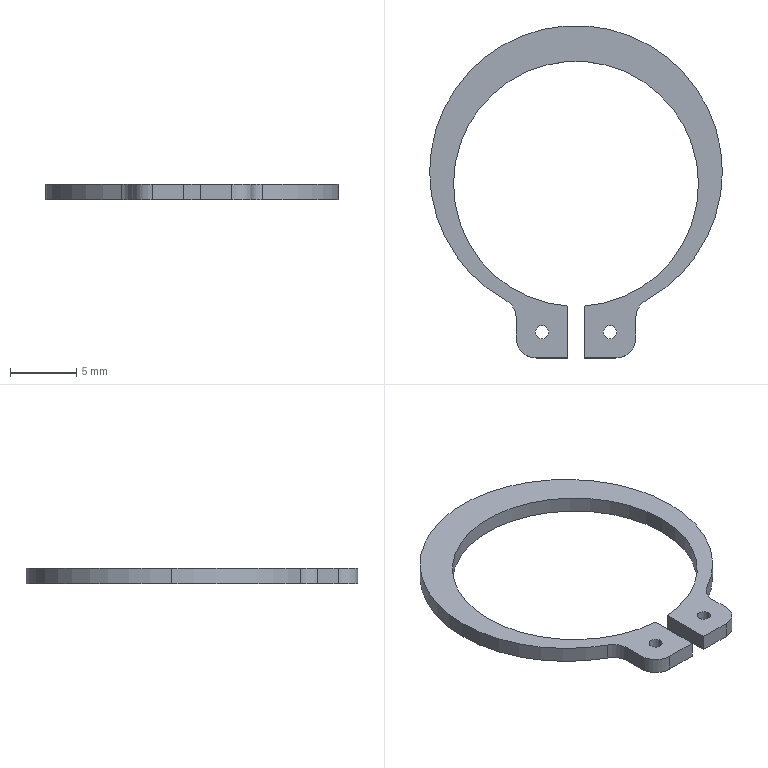Part | NX | features BREP 1 | 1 solid | 22 faces | box 22.1 x 25.1 x 1.2 mm | volume 165.202 mm3 | cylinder 14 | plane 8 | commonest cylinder face diameters 1 x4 3.011 x4 18.5 x3 22.1 x3
STEP:
#1=CARTESIAN_POINT('',(-3.067,-11.2,0.6));
#2=VERTEX_POINT('',#1);
#3=CARTESIAN_POINT('',(-2.067,-11.2,0.6));
#4=VERTEX_POINT('',#3);
#5=CARTESIAN_POINT('',(-2.567,-11.2,0.6));
#6=DIRECTION('',(0.,0.,1.));
#7=DIRECTION('',(1.,0.,0.));
#8=AXIS2_PLACEMENT_3D('',#5,#6,#7);
#9=CIRCLE('',#8,0.5);
#10=EDGE_CURVE('',#2,#4,#9,.T.);
#11=ORIENTED_EDGE('',*,*,#10,.T.);
#12=CARTESIAN_POINT('',(-2.067,-11.2,-0.6));
#13=VERTEX_POINT('',#12);
#14=CARTESIAN_POINT('',(-2.067,-11.2,0.6));
#15=DIRECTION('',(0.,0.,-1.));
#16=VECTOR('',#15,1000.);
#17=LINE('',#14,#16);
#18=EDGE_CURVE('',#13,#4,#17,.F.);
#19=ORIENTED_EDGE('',*,*,#18,.F.);
#20=CARTESIAN_POINT('',(-3.067,-11.2,-0.6));
#21=VERTEX_POINT('',#20);
#22=CARTESIAN_POINT('',(-2.567,-11.2,-0.6));
#23=DIRECTION('',(0.,0.,1.));
#24=DIRECTION('',(1.,0.,0.));
#25=AXIS2_PLACEMENT_3D('',#22,#23,#24);
#26=CIRCLE('',#25,0.5);
#27=EDGE_CURVE('',#21,#13,#26,.T.);
#28=ORIENTED_EDGE('',*,*,#27,.F.);
#29=CARTESIAN_POINT('',(-3.067,-11.2,0.6));
#30=DIRECTION('',(0.,0.,-1.));
#31=VECTOR('',#30,1000.);
#32=LINE('',#29,#31);
#33=EDGE_CURVE('',#21,#2,#32,.F.);
#34=ORIENTED_EDGE('',*,*,#33,.T.);
#35=EDGE_LOOP('',(#11,#19,#28,#34));
#36=FACE_BOUND('',#35,.T.);
#37=CARTESIAN_POINT('',(-2.567,-11.2,0.6));
#38=DIRECTION('',(0.,0.,-1.));
#39=DIRECTION('',(1.,0.,0.));
#40=AXIS2_PLACEMENT_3D('',#37,#38,#39);
#41=CYLINDRICAL_SURFACE('',#40,0.5);
#42=ADVANCED_FACE('',(#36),#41,.F.);
#43=CARTESIAN_POINT('',(2.067,-11.2,0.6));
#44=VERTEX_POINT('',#43);
#45=CARTESIAN_POINT('',(3.067,-11.2,0.6));
#46=VERTEX_POINT('',#45);
#47=CARTESIAN_POINT('',(2.567,-11.2,0.6));
#48=DIRECTION('',(0.,0.,1.));
#49=DIRECTION('',(1.,0.,0.));
#50=AXIS2_PLACEMENT_3D('',#47,#48,#49);
#51=CIRCLE('',#50,0.5);
#52=EDGE_CURVE('',#44,#46,#51,.T.);
#53=ORIENTED_EDGE('',*,*,#52,.T.);
#54=CARTESIAN_POINT('',(3.067,-11.2,-0.6));
#55=VERTEX_POINT('',#54);
#56=CARTESIAN_POINT('',(3.067,-11.2,0.6));
#57=DIRECTION('',(0.,0.,-1.));
#58=VECTOR('',#57,1000.);
#59=LINE('',#56,#58);
#60=EDGE_CURVE('',#55,#46,#59,.F.);
#61=ORIENTED_EDGE('',*,*,#60,.F.);
#62=CARTESIAN_POINT('',(2.067,-11.2,-0.6));
#63=VERTEX_POINT('',#62);
#64=CARTESIAN_POINT('',(2.567,-11.2,-0.6));
#65=DIRECTION('',(0.,0.,1.));
#66=DIRECTION('',(1.,0.,0.));
#67=AXIS2_PLACEMENT_3D('',#64,#65,#66);
#68=CIRCLE('',#67,0.5);
#69=EDGE_CURVE('',#63,#55,#68,.T.);
#70=ORIENTED_EDGE('',*,*,#69,.F.);
#71=CARTESIAN_POINT('',(2.067,-11.2,0.6));
#72=DIRECTION('',(0.,0.,-1.));
#73=VECTOR('',#72,1000.);
#74=LINE('',#71,#73);
#75=EDGE_CURVE('',#63,#44,#74,.F.);
#76=ORIENTED_EDGE('',*,*,#75,.T.);
#77=EDGE_LOOP('',(#53,#61,#70,#76));
#78=FACE_BOUND('',#77,.T.);
#79=CARTESIAN_POINT('',(2.567,-11.2,0.6));
#80=DIRECTION('',(0.,0.,-1.));
#81=DIRECTION('',(1.,0.,0.));
#82=AXIS2_PLACEMENT_3D('',#79,#80,#81);
#83=CYLINDRICAL_SURFACE('',#82,0.5);
#84=ADVANCED_FACE('',(#78),#83,.F.);
#85=CARTESIAN_POINT('',(9.25,0.,0.6));
#86=VERTEX_POINT('',#85);
#87=CARTESIAN_POINT('',(0.6167,-9.229,0.6));
#88=VERTEX_POINT('',#87);
#89=CARTESIAN_POINT('',(0.,0.,0.6));
#90=DIRECTION('',(0.,0.,-1.));
#91=DIRECTION('',(-1.,0.,0.));
#92=AXIS2_PLACEMENT_3D('',#89,#90,#91);
#93=CIRCLE('',#92,9.25);
#94=EDGE_CURVE('',#86,#88,#93,.T.);
#95=ORIENTED_EDGE('',*,*,#94,.F.);
#96=CARTESIAN_POINT('',(9.25,0.,-0.6));
#97=VERTEX_POINT('',#96);
#98=CARTESIAN_POINT('',(9.25,0.,0.6));
#99=DIRECTION('',(0.,0.,-1.));
#100=VECTOR('',#99,1000.);
#101=LINE('',#98,#100);
#102=EDGE_CURVE('',#86,#97,#101,.T.);
#103=ORIENTED_EDGE('',*,*,#102,.T.);
#104=CARTESIAN_POINT('',(0.6167,-9.229,-0.6));
#105=VERTEX_POINT('',#104);
#106=CARTESIAN_POINT('',(0.,0.,-0.6));
#107=DIRECTION('',(0.,0.,-1.));
#108=DIRECTION('',(-1.,0.,0.));
#109=AXIS2_PLACEMENT_3D('',#106,#107,#108);
#110=CIRCLE('',#109,9.25);
#111=EDGE_CURVE('',#97,#105,#110,.T.);
#112=ORIENTED_EDGE('',*,*,#111,.T.);
#113=CARTESIAN_POINT('',(0.6167,-9.229,0.6));
#114=DIRECTION('',(0.,0.,-1.));
#115=VECTOR('',#114,1000.);
#116=LINE('',#113,#115);
#117=EDGE_CURVE('',#88,#105,#116,.T.);
#118=ORIENTED_EDGE('',*,*,#117,.F.);
#119=EDGE_LOOP('',(#95,#103,#112,#118));
#120=FACE_BOUND('',#119,.T.);
#121=CARTESIAN_POINT('',(0.,0.,0.6));
#122=DIRECTION('',(0.,0.,-1.));
#123=DIRECTION('',(1.,0.,0.));
#124=AXIS2_PLACEMENT_3D('',#121,#122,#123);
#125=CYLINDRICAL_SURFACE('',#124,9.25);
#126=ADVANCED_FACE('',(#120),#125,.F.);
#127=ORIENTED_EDGE('',*,*,#102,.F.);
#128=CARTESIAN_POINT('',(-9.25,0.,0.6));
#129=VERTEX_POINT('',#128);
#130=CARTESIAN_POINT('',(0.,0.,0.6));
#131=DIRECTION('',(0.,0.,-1.));
#132=DIRECTION('',(-1.,0.,0.));
#133=AXIS2_PLACEMENT_3D('',#130,#131,#132);
#134=CIRCLE('',#133,9.25);
#135=EDGE_CURVE('',#129,#86,#134,.T.);
#136=ORIENTED_EDGE('',*,*,#135,.F.);
#137=CARTESIAN_POINT('',(-9.25,0.,-0.6));
#138=VERTEX_POINT('',#137);
#139=CARTESIAN_POINT('',(-9.25,0.,0.6));
#140=DIRECTION('',(0.,0.,-1.));
#141=VECTOR('',#140,1000.);
#142=LINE('',#139,#141);
#143=EDGE_CURVE('',#129,#138,#142,.T.);
#144=ORIENTED_EDGE('',*,*,#143,.T.);
#145=CARTESIAN_POINT('',(0.,0.,-0.6));
#146=DIRECTION('',(0.,0.,-1.));
#147=DIRECTION('',(-1.,0.,0.));
#148=AXIS2_PLACEMENT_3D('',#145,#146,#147);
#149=CIRCLE('',#148,9.25);
#150=EDGE_CURVE('',#138,#97,#149,.T.);
#151=ORIENTED_EDGE('',*,*,#150,.T.);
#152=EDGE_LOOP('',(#127,#136,#144,#151));
#153=FACE_BOUND('',#152,.T.);
#154=CARTESIAN_POINT('',(0.,0.,0.6));
#155=DIRECTION('',(0.,0.,-1.));
#156=DIRECTION('',(1.,0.,0.));
#157=AXIS2_PLACEMENT_3D('',#154,#155,#156);
#158=CYLINDRICAL_SURFACE('',#157,9.25);
#159=ADVANCED_FACE('',(#153),#158,.F.);
#160=CARTESIAN_POINT('',(11.05,0.9,0.6));
#161=VERTEX_POINT('',#160);
#162=CARTESIAN_POINT('',(-11.05,0.9,0.6));
#163=VERTEX_POINT('',#162);
#164=CARTESIAN_POINT('',(0.,0.9,0.6));
#165=DIRECTION('',(0.,0.,1.));
#166=DIRECTION('',(1.,0.,0.));
#167=AXIS2_PLACEMENT_3D('',#164,#165,#166);
#168=CIRCLE('',#167,11.05);
#169=EDGE_CURVE('',#161,#163,#168,.T.);
#170=ORIENTED_EDGE('',*,*,#169,.F.);
#171=CARTESIAN_POINT('',(11.05,0.9,-0.6));
#172=VERTEX_POINT('',#171);
#173=CARTESIAN_POINT('',(11.05,0.9,0.6));
#174=DIRECTION('',(0.,0.,-1.));
#175=VECTOR('',#174,1000.);
#176=LINE('',#173,#175);
#177=EDGE_CURVE('',#161,#172,#176,.T.);
#178=ORIENTED_EDGE('',*,*,#177,.T.);
#179=CARTESIAN_POINT('',(-11.05,0.9,-0.6));
#180=VERTEX_POINT('',#179);
#181=CARTESIAN_POINT('',(0.,0.9,-0.6));
#182=DIRECTION('',(0.,0.,1.));
#183=DIRECTION('',(1.,0.,0.));
#184=AXIS2_PLACEMENT_3D('',#181,#182,#183);
#185=CIRCLE('',#184,11.05);
#186=EDGE_CURVE('',#172,#180,#185,.T.);
#187=ORIENTED_EDGE('',*,*,#186,.T.);
#188=CARTESIAN_POINT('',(-11.05,0.9,0.6));
#189=DIRECTION('',(0.,0.,-1.));
#190=VECTOR('',#189,1000.);
#191=LINE('',#188,#190);
#192=EDGE_CURVE('',#163,#180,#191,.T.);
#193=ORIENTED_EDGE('',*,*,#192,.F.);
#194=EDGE_LOOP('',(#170,#178,#187,#193));
#195=FACE_BOUND('',#194,.T.);
#196=CARTESIAN_POINT('',(0.,0.9,0.6));
#197=DIRECTION('',(0.,0.,-1.));
#198=DIRECTION('',(1.,0.,0.));
#199=AXIS2_PLACEMENT_3D('',#196,#197,#198);
#200=CYLINDRICAL_SURFACE('',#199,11.05);
#201=ADVANCED_FACE('',(#195),#200,.T.);
#202=CARTESIAN_POINT('',(-5.3,-8.796,0.6));
#203=VERTEX_POINT('',#202);
#204=CARTESIAN_POINT('',(0.,0.9,0.6));
#205=DIRECTION('',(0.,0.,1.));
#206=DIRECTION('',(1.,0.,0.));
#207=AXIS2_PLACEMENT_3D('',#204,#205,#206);
#208=CIRCLE('',#207,11.05);
#209=EDGE_CURVE('',#163,#203,#208,.T.);
#210=ORIENTED_EDGE('',*,*,#209,.F.);
#211=ORIENTED_EDGE('',*,*,#192,.T.);
#212=CARTESIAN_POINT('',(-5.3,-8.796,-0.6));
#213=VERTEX_POINT('',#212);
#214=CARTESIAN_POINT('',(0.,0.9,-0.6));
#215=DIRECTION('',(0.,0.,1.));
#216=DIRECTION('',(1.,0.,0.));
#217=AXIS2_PLACEMENT_3D('',#214,#215,#216);
#218=CIRCLE('',#217,11.05);
#219=EDGE_CURVE('',#180,#213,#218,.T.);
#220=ORIENTED_EDGE('',*,*,#219,.T.);
#221=CARTESIAN_POINT('',(-5.3,-8.796,0.6));
#222=DIRECTION('',(0.,0.,-1.));
#223=VECTOR('',#222,1000.);
#224=LINE('',#221,#223);
#225=EDGE_CURVE('',#203,#213,#224,.T.);
#226=ORIENTED_EDGE('',*,*,#225,.F.);
#227=EDGE_LOOP('',(#210,#211,#220,#226));
#228=FACE_BOUND('',#227,.T.);
#229=CARTESIAN_POINT('',(0.,0.9,0.6));
#230=DIRECTION('',(0.,0.,-1.));
#231=DIRECTION('',(1.,0.,0.));
#232=AXIS2_PLACEMENT_3D('',#229,#230,#231);
#233=CYLINDRICAL_SURFACE('',#232,11.05);
#234=ADVANCED_FACE('',(#228),#233,.T.);
#235=CARTESIAN_POINT('',(4.517,-10.117,0.6));
#236=VERTEX_POINT('',#235);
#237=CARTESIAN_POINT('',(5.3,-8.796,0.6));
#238=VERTEX_POINT('',#237);
#239=CARTESIAN_POINT('',(6.022,-10.117,0.6));
#240=DIRECTION('',(0.,0.,-1.));
#241=DIRECTION('',(-1.,0.,0.));
#242=AXIS2_PLACEMENT_3D('',#239,#240,#241);
#243=CIRCLE('',#242,1.506);
#244=EDGE_CURVE('',#236,#238,#243,.T.);
#245=ORIENTED_EDGE('',*,*,#244,.T.);
#246=CARTESIAN_POINT('',(0.,0.9,0.6));
#247=DIRECTION('',(0.,0.,1.));
#248=DIRECTION('',(1.,0.,0.));
#249=AXIS2_PLACEMENT_3D('',#246,#247,#248);
#250=CIRCLE('',#249,11.05);
#251=EDGE_CURVE('',#238,#161,#250,.T.);
#252=ORIENTED_EDGE('',*,*,#251,.T.);
#253=ORIENTED_EDGE('',*,*,#169,.T.);
#254=ORIENTED_EDGE('',*,*,#209,.T.);
#255=CARTESIAN_POINT('',(-4.517,-10.117,0.6));
#256=VERTEX_POINT('',#255);
#257=CARTESIAN_POINT('',(-6.022,-10.117,0.6));
#258=DIRECTION('',(0.,0.,-1.));
#259=DIRECTION('',(-1.,0.,0.));
#260=AXIS2_PLACEMENT_3D('',#257,#258,#259);
#261=CIRCLE('',#260,1.506);
#262=EDGE_CURVE('',#203,#256,#261,.T.);
#263=ORIENTED_EDGE('',*,*,#262,.T.);
#264=CARTESIAN_POINT('',(-4.517,-11.644,0.6));
#265=VERTEX_POINT('',#264);
#266=CARTESIAN_POINT('',(-4.517,-10.117,0.6));
#267=DIRECTION('',(0.,-1.,0.));
#268=VECTOR('',#267,1000.);
#269=LINE('',#266,#268);
#270=EDGE_CURVE('',#256,#265,#269,.T.);
#271=ORIENTED_EDGE('',*,*,#270,.T.);
#272=CARTESIAN_POINT('',(-3.011,-13.15,0.6));
#273=VERTEX_POINT('',#272);
#274=CARTESIAN_POINT('',(-3.011,-11.644,0.6));
#275=DIRECTION('',(0.,0.,1.));
#276=DIRECTION('',(1.,0.,0.));
#277=AXIS2_PLACEMENT_3D('',#274,#275,#276);
#278=CIRCLE('',#277,1.506);
#279=EDGE_CURVE('',#265,#273,#278,.T.);
#280=ORIENTED_EDGE('',*,*,#279,.T.);
#281=CARTESIAN_POINT('',(-0.6167,-13.15,0.6));
#282=VERTEX_POINT('',#281);
#283=CARTESIAN_POINT('',(-3.011,-13.15,0.6));
#284=DIRECTION('',(1.,0.,0.));
#285=VECTOR('',#284,1000.);
#286=LINE('',#283,#285);
#287=EDGE_CURVE('',#273,#282,#286,.T.);
#288=ORIENTED_EDGE('',*,*,#287,.T.);
#289=CARTESIAN_POINT('',(-0.6167,-9.229,0.6));
#290=VERTEX_POINT('',#289);
#291=CARTESIAN_POINT('',(-0.6167,-13.15,0.6));
#292=DIRECTION('',(0.,1.,0.));
#293=VECTOR('',#292,1000.);
#294=LINE('',#291,#293);
#295=EDGE_CURVE('',#282,#290,#294,.T.);
#296=ORIENTED_EDGE('',*,*,#295,.T.);
#297=CARTESIAN_POINT('',(0.,0.,0.6));
#298=DIRECTION('',(0.,0.,-1.));
#299=DIRECTION('',(-1.,0.,0.));
#300=AXIS2_PLACEMENT_3D('',#297,#298,#299);
#301=CIRCLE('',#300,9.25);
#302=EDGE_CURVE('',#290,#129,#301,.T.);
#303=ORIENTED_EDGE('',*,*,#302,.T.);
#304=ORIENTED_EDGE('',*,*,#135,.T.);
#305=ORIENTED_EDGE('',*,*,#94,.T.);
#306=CARTESIAN_POINT('',(0.6167,-13.15,0.6));
#307=VERTEX_POINT('',#306);
#308=CARTESIAN_POINT('',(0.6167,-9.229,0.6));
#309=DIRECTION('',(0.,-1.,0.));
#310=VECTOR('',#309,1000.);
#311=LINE('',#308,#310);
#312=EDGE_CURVE('',#88,#307,#311,.T.);
#313=ORIENTED_EDGE('',*,*,#312,.T.);
#314=CARTESIAN_POINT('',(3.011,-13.15,0.6));
#315=VERTEX_POINT('',#314);
#316=CARTESIAN_POINT('',(0.6167,-13.15,0.6));
#317=DIRECTION('',(1.,0.,0.));
#318=VECTOR('',#317,1000.);
#319=LINE('',#316,#318);
#320=EDGE_CURVE('',#307,#315,#319,.T.);
#321=ORIENTED_EDGE('',*,*,#320,.T.);
#322=CARTESIAN_POINT('',(4.517,-11.644,0.6));
#323=VERTEX_POINT('',#322);
#324=CARTESIAN_POINT('',(3.011,-11.644,0.6));
#325=DIRECTION('',(0.,0.,1.));
#326=DIRECTION('',(1.,0.,0.));
#327=AXIS2_PLACEMENT_3D('',#324,#325,#326);
#328=CIRCLE('',#327,1.506);
#329=EDGE_CURVE('',#315,#323,#328,.T.);
#330=ORIENTED_EDGE('',*,*,#329,.T.);
#331=CARTESIAN_POINT('',(4.517,-11.644,0.6));
#332=DIRECTION('',(0.,1.,0.));
#333=VECTOR('',#332,1000.);
#334=LINE('',#331,#333);
#335=EDGE_CURVE('',#323,#236,#334,.T.);
#336=ORIENTED_EDGE('',*,*,#335,.T.);
#337=EDGE_LOOP('',(#245,#252,#253,#254,#263,#271,#280,#288,#296,#303,#304,#305,#313,#321,#330,#336));
#338=FACE_BOUND('',#337,.T.);
#339=ORIENTED_EDGE('',*,*,#52,.F.);
#340=CARTESIAN_POINT('',(2.567,-11.2,0.6));
#341=DIRECTION('',(0.,0.,1.));
#342=DIRECTION('',(1.,0.,0.));
#343=AXIS2_PLACEMENT_3D('',#340,#341,#342);
#344=CIRCLE('',#343,0.5);
#345=EDGE_CURVE('',#46,#44,#344,.T.);
#346=ORIENTED_EDGE('',*,*,#345,.F.);
#347=EDGE_LOOP('',(#339,#346));
#348=FACE_BOUND('',#347,.T.);
#349=ORIENTED_EDGE('',*,*,#10,.F.);
#350=CARTESIAN_POINT('',(-2.567,-11.2,0.6));
#351=DIRECTION('',(0.,0.,1.));
#352=DIRECTION('',(1.,0.,0.));
#353=AXIS2_PLACEMENT_3D('',#350,#351,#352);
#354=CIRCLE('',#353,0.5);
#355=EDGE_CURVE('',#4,#2,#354,.T.);
#356=ORIENTED_EDGE('',*,*,#355,.F.);
#357=EDGE_LOOP('',(#349,#356));
#358=FACE_BOUND('',#357,.T.);
#359=CARTESIAN_POINT('',(6.022,-10.117,0.6));
#360=DIRECTION('',(0.,0.,-1.));
#361=DIRECTION('',(1.,0.,0.));
#362=AXIS2_PLACEMENT_3D('',#359,#360,#361);
#363=PLANE('',#362);
#364=ADVANCED_FACE('',(#338,#348,#358),#363,.F.);
#365=CARTESIAN_POINT('',(4.517,-10.117,-0.6));
#366=VERTEX_POINT('',#365);
#367=CARTESIAN_POINT('',(4.517,-10.117,0.6));
#368=DIRECTION('',(0.,0.,-1.));
#369=VECTOR('',#368,1000.);
#370=LINE('',#367,#369);
#371=EDGE_CURVE('',#236,#366,#370,.T.);
#372=ORIENTED_EDGE('',*,*,#371,.T.);
#373=CARTESIAN_POINT('',(5.3,-8.796,-0.6));
#374=VERTEX_POINT('',#373);
#375=CARTESIAN_POINT('',(6.022,-10.117,-0.6));
#376=DIRECTION('',(0.,0.,-1.));
#377=DIRECTION('',(-1.,0.,0.));
#378=AXIS2_PLACEMENT_3D('',#375,#376,#377);
#379=CIRCLE('',#378,1.506);
#380=EDGE_CURVE('',#366,#374,#379,.T.);
#381=ORIENTED_EDGE('',*,*,#380,.T.);
#382=CARTESIAN_POINT('',(5.3,-8.796,0.6));
#383=DIRECTION('',(0.,0.,-1.));
#384=VECTOR('',#383,1000.);
#385=LINE('',#382,#384);
#386=EDGE_CURVE('',#238,#374,#385,.T.);
#387=ORIENTED_EDGE('',*,*,#386,.F.);
#388=ORIENTED_EDGE('',*,*,#244,.F.);
#389=EDGE_LOOP('',(#372,#381,#387,#388));
#390=FACE_BOUND('',#389,.T.);
#391=CARTESIAN_POINT('',(6.022,-10.117,0.6));
#392=DIRECTION('',(0.,0.,-1.));
#393=DIRECTION('',(1.,0.,0.));
#394=AXIS2_PLACEMENT_3D('',#391,#392,#393);
#395=CYLINDRICAL_SURFACE('',#394,1.506);
#396=ADVANCED_FACE('',(#390),#395,.F.);
#397=ORIENTED_EDGE('',*,*,#177,.F.);
#398=ORIENTED_EDGE('',*,*,#251,.F.);
#399=ORIENTED_EDGE('',*,*,#386,.T.);
#400=CARTESIAN_POINT('',(0.,0.9,-0.6));
#401=DIRECTION('',(0.,0.,1.));
#402=DIRECTION('',(1.,0.,0.));
#403=AXIS2_PLACEMENT_3D('',#400,#401,#402);
#404=CIRCLE('',#403,11.05);
#405=EDGE_CURVE('',#374,#172,#404,.T.);
#406=ORIENTED_EDGE('',*,*,#405,.T.);
#407=EDGE_LOOP('',(#397,#398,#399,#406));
#408=FACE_BOUND('',#407,.T.);
#409=CARTESIAN_POINT('',(0.,0.9,0.6));
#410=DIRECTION('',(0.,0.,-1.));
#411=DIRECTION('',(1.,0.,0.));
#412=AXIS2_PLACEMENT_3D('',#409,#410,#411);
#413=CYLINDRICAL_SURFACE('',#412,11.05);
#414=ADVANCED_FACE('',(#408),#413,.T.);
#415=ORIENTED_EDGE('',*,*,#225,.T.);
#416=CARTESIAN_POINT('',(-4.517,-10.117,-0.6));
#417=VERTEX_POINT('',#416);
#418=CARTESIAN_POINT('',(-6.022,-10.117,-0.6));
#419=DIRECTION('',(0.,0.,-1.));
#420=DIRECTION('',(-1.,0.,0.));
#421=AXIS2_PLACEMENT_3D('',#418,#419,#420);
#422=CIRCLE('',#421,1.506);
#423=EDGE_CURVE('',#213,#417,#422,.T.);
#424=ORIENTED_EDGE('',*,*,#423,.T.);
#425=CARTESIAN_POINT('',(-4.517,-10.117,0.6));
#426=DIRECTION('',(0.,0.,-1.));
#427=VECTOR('',#426,1000.);
#428=LINE('',#425,#427);
#429=EDGE_CURVE('',#256,#417,#428,.T.);
#430=ORIENTED_EDGE('',*,*,#429,.F.);
#431=ORIENTED_EDGE('',*,*,#262,.F.);
#432=EDGE_LOOP('',(#415,#424,#430,#431));
#433=FACE_BOUND('',#432,.T.);
#434=CARTESIAN_POINT('',(-6.022,-10.117,0.6));
#435=DIRECTION('',(0.,0.,-1.));
#436=DIRECTION('',(1.,0.,0.));
#437=AXIS2_PLACEMENT_3D('',#434,#435,#436);
#438=CYLINDRICAL_SURFACE('',#437,1.506);
#439=ADVANCED_FACE('',(#433),#438,.F.);
#440=ORIENTED_EDGE('',*,*,#429,.T.);
#441=CARTESIAN_POINT('',(-4.517,-11.644,-0.6));
#442=VERTEX_POINT('',#441);
#443=CARTESIAN_POINT('',(-4.517,-10.117,-0.6));
#444=DIRECTION('',(0.,-1.,0.));
#445=VECTOR('',#444,1000.);
#446=LINE('',#443,#445);
#447=EDGE_CURVE('',#417,#442,#446,.T.);
#448=ORIENTED_EDGE('',*,*,#447,.T.);
#449=CARTESIAN_POINT('',(-4.517,-11.644,0.6));
#450=DIRECTION('',(0.,0.,-1.));
#451=VECTOR('',#450,1000.);
#452=LINE('',#449,#451);
#453=EDGE_CURVE('',#265,#442,#452,.T.);
#454=ORIENTED_EDGE('',*,*,#453,.F.);
#455=ORIENTED_EDGE('',*,*,#270,.F.);
#456=EDGE_LOOP('',(#440,#448,#454,#455));
#457=FACE_BOUND('',#456,.T.);
#458=CARTESIAN_POINT('',(-4.517,-10.117,0.6));
#459=DIRECTION('',(1.,0.,0.));
#460=DIRECTION('',(0.,0.,1.));
#461=AXIS2_PLACEMENT_3D('',#458,#459,#460);
#462=PLANE('',#461);
#463=ADVANCED_FACE('',(#457),#462,.F.);
#464=ORIENTED_EDGE('',*,*,#453,.T.);
#465=CARTESIAN_POINT('',(-3.011,-13.15,-0.6));
#466=VERTEX_POINT('',#465);
#467=CARTESIAN_POINT('',(-3.011,-11.644,-0.6));
#468=DIRECTION('',(0.,0.,1.));
#469=DIRECTION('',(1.,0.,0.));
#470=AXIS2_PLACEMENT_3D('',#467,#468,#469);
#471=CIRCLE('',#470,1.506);
#472=EDGE_CURVE('',#442,#466,#471,.T.);
#473=ORIENTED_EDGE('',*,*,#472,.T.);
#474=CARTESIAN_POINT('',(-3.011,-13.15,0.6));
#475=DIRECTION('',(0.,0.,-1.));
#476=VECTOR('',#475,1000.);
#477=LINE('',#474,#476);
#478=EDGE_CURVE('',#273,#466,#477,.T.);
#479=ORIENTED_EDGE('',*,*,#478,.F.);
#480=ORIENTED_EDGE('',*,*,#279,.F.);
#481=EDGE_LOOP('',(#464,#473,#479,#480));
#482=FACE_BOUND('',#481,.T.);
#483=CARTESIAN_POINT('',(-3.011,-11.644,0.6));
#484=DIRECTION('',(0.,0.,-1.));
#485=DIRECTION('',(1.,0.,0.));
#486=AXIS2_PLACEMENT_3D('',#483,#484,#485);
#487=CYLINDRICAL_SURFACE('',#486,1.506);
#488=ADVANCED_FACE('',(#482),#487,.T.);
#489=ORIENTED_EDGE('',*,*,#478,.T.);
#490=CARTESIAN_POINT('',(-0.6167,-13.15,-0.6));
#491=VERTEX_POINT('',#490);
#492=CARTESIAN_POINT('',(-3.011,-13.15,-0.6));
#493=DIRECTION('',(1.,0.,0.));
#494=VECTOR('',#493,1000.);
#495=LINE('',#492,#494);
#496=EDGE_CURVE('',#466,#491,#495,.T.);
#497=ORIENTED_EDGE('',*,*,#496,.T.);
#498=CARTESIAN_POINT('',(-0.6167,-13.15,0.6));
#499=DIRECTION('',(0.,0.,-1.));
#500=VECTOR('',#499,1000.);
#501=LINE('',#498,#500);
#502=EDGE_CURVE('',#282,#491,#501,.T.);
#503=ORIENTED_EDGE('',*,*,#502,.F.);
#504=ORIENTED_EDGE('',*,*,#287,.F.);
#505=EDGE_LOOP('',(#489,#497,#503,#504));
#506=FACE_BOUND('',#505,.T.);
#507=CARTESIAN_POINT('',(-3.011,-13.15,0.6));
#508=DIRECTION('',(0.,1.,0.));
#509=DIRECTION('',(0.,0.,-1.));
#510=AXIS2_PLACEMENT_3D('',#507,#508,#509);
#511=PLANE('',#510);
#512=ADVANCED_FACE('',(#506),#511,.F.);
#513=ORIENTED_EDGE('',*,*,#502,.T.);
#514=CARTESIAN_POINT('',(-0.6167,-9.229,-0.6));
#515=VERTEX_POINT('',#514);
#516=CARTESIAN_POINT('',(-0.6167,-13.15,-0.6));
#517=DIRECTION('',(0.,1.,0.));
#518=VECTOR('',#517,1000.);
#519=LINE('',#516,#518);
#520=EDGE_CURVE('',#491,#515,#519,.T.);
#521=ORIENTED_EDGE('',*,*,#520,.T.);
#522=CARTESIAN_POINT('',(-0.6167,-9.229,0.6));
#523=DIRECTION('',(0.,0.,-1.));
#524=VECTOR('',#523,1000.);
#525=LINE('',#522,#524);
#526=EDGE_CURVE('',#290,#515,#525,.T.);
#527=ORIENTED_EDGE('',*,*,#526,.F.);
#528=ORIENTED_EDGE('',*,*,#295,.F.);
#529=EDGE_LOOP('',(#513,#521,#527,#528));
#530=FACE_BOUND('',#529,.T.);
#531=CARTESIAN_POINT('',(-0.6167,-13.15,0.6));
#532=DIRECTION('',(-1.,0.,0.));
#533=DIRECTION('',(0.,0.,-1.));
#534=AXIS2_PLACEMENT_3D('',#531,#532,#533);
#535=PLANE('',#534);
#536=ADVANCED_FACE('',(#530),#535,.F.);
#537=ORIENTED_EDGE('',*,*,#143,.F.);
#538=ORIENTED_EDGE('',*,*,#302,.F.);
#539=ORIENTED_EDGE('',*,*,#526,.T.);
#540=CARTESIAN_POINT('',(0.,0.,-0.6));
#541=DIRECTION('',(0.,0.,-1.));
#542=DIRECTION('',(-1.,0.,0.));
#543=AXIS2_PLACEMENT_3D('',#540,#541,#542);
#544=CIRCLE('',#543,9.25);
#545=EDGE_CURVE('',#515,#138,#544,.T.);
#546=ORIENTED_EDGE('',*,*,#545,.T.);
#547=EDGE_LOOP('',(#537,#538,#539,#546));
#548=FACE_BOUND('',#547,.T.);
#549=CARTESIAN_POINT('',(0.,0.,0.6));
#550=DIRECTION('',(0.,0.,-1.));
#551=DIRECTION('',(1.,0.,0.));
#552=AXIS2_PLACEMENT_3D('',#549,#550,#551);
#553=CYLINDRICAL_SURFACE('',#552,9.25);
#554=ADVANCED_FACE('',(#548),#553,.F.);
#555=ORIENTED_EDGE('',*,*,#117,.T.);
#556=CARTESIAN_POINT('',(0.6167,-13.15,-0.6));
#557=VERTEX_POINT('',#556);
#558=CARTESIAN_POINT('',(0.6167,-9.229,-0.6));
#559=DIRECTION('',(0.,-1.,0.));
#560=VECTOR('',#559,1000.);
#561=LINE('',#558,#560);
#562=EDGE_CURVE('',#105,#557,#561,.T.);
#563=ORIENTED_EDGE('',*,*,#562,.T.);
#564=CARTESIAN_POINT('',(0.6167,-13.15,0.6));
#565=DIRECTION('',(0.,0.,-1.));
#566=VECTOR('',#565,1000.);
#567=LINE('',#564,#566);
#568=EDGE_CURVE('',#307,#557,#567,.T.);
#569=ORIENTED_EDGE('',*,*,#568,.F.);
#570=ORIENTED_EDGE('',*,*,#312,.F.);
#571=EDGE_LOOP('',(#555,#563,#569,#570));
#572=FACE_BOUND('',#571,.T.);
#573=CARTESIAN_POINT('',(0.6167,-9.229,0.6));
#574=DIRECTION('',(1.,0.,0.));
#575=DIRECTION('',(0.,0.,1.));
#576=AXIS2_PLACEMENT_3D('',#573,#574,#575);
#577=PLANE('',#576);
#578=ADVANCED_FACE('',(#572),#577,.F.);
#579=ORIENTED_EDGE('',*,*,#568,.T.);
#580=CARTESIAN_POINT('',(3.011,-13.15,-0.6));
#581=VERTEX_POINT('',#580);
#582=CARTESIAN_POINT('',(0.6167,-13.15,-0.6));
#583=DIRECTION('',(1.,0.,0.));
#584=VECTOR('',#583,1000.);
#585=LINE('',#582,#584);
#586=EDGE_CURVE('',#557,#581,#585,.T.);
#587=ORIENTED_EDGE('',*,*,#586,.T.);
#588=CARTESIAN_POINT('',(3.011,-13.15,0.6));
#589=DIRECTION('',(0.,0.,-1.));
#590=VECTOR('',#589,1000.);
#591=LINE('',#588,#590);
#592=EDGE_CURVE('',#315,#581,#591,.T.);
#593=ORIENTED_EDGE('',*,*,#592,.F.);
#594=ORIENTED_EDGE('',*,*,#320,.F.);
#595=EDGE_LOOP('',(#579,#587,#593,#594));
#596=FACE_BOUND('',#595,.T.);
#597=CARTESIAN_POINT('',(0.6167,-13.15,0.6));
#598=DIRECTION('',(0.,1.,0.));
#599=DIRECTION('',(0.,0.,-1.));
#600=AXIS2_PLACEMENT_3D('',#597,#598,#599);
#601=PLANE('',#600);
#602=ADVANCED_FACE('',(#596),#601,.F.);
#603=ORIENTED_EDGE('',*,*,#592,.T.);
#604=CARTESIAN_POINT('',(4.517,-11.644,-0.6));
#605=VERTEX_POINT('',#604);
#606=CARTESIAN_POINT('',(3.011,-11.644,-0.6));
#607=DIRECTION('',(0.,0.,1.));
#608=DIRECTION('',(1.,0.,0.));
#609=AXIS2_PLACEMENT_3D('',#606,#607,#608);
#610=CIRCLE('',#609,1.506);
#611=EDGE_CURVE('',#581,#605,#610,.T.);
#612=ORIENTED_EDGE('',*,*,#611,.T.);
#613=CARTESIAN_POINT('',(4.517,-11.644,0.6));
#614=DIRECTION('',(0.,0.,-1.));
#615=VECTOR('',#614,1000.);
#616=LINE('',#613,#615);
#617=EDGE_CURVE('',#323,#605,#616,.T.);
#618=ORIENTED_EDGE('',*,*,#617,.F.);
#619=ORIENTED_EDGE('',*,*,#329,.F.);
#620=EDGE_LOOP('',(#603,#612,#618,#619));
#621=FACE_BOUND('',#620,.T.);
#622=CARTESIAN_POINT('',(3.011,-11.644,0.6));
#623=DIRECTION('',(0.,0.,-1.));
#624=DIRECTION('',(1.,0.,0.));
#625=AXIS2_PLACEMENT_3D('',#622,#623,#624);
#626=CYLINDRICAL_SURFACE('',#625,1.506);
#627=ADVANCED_FACE('',(#621),#626,.T.);
#628=ORIENTED_EDGE('',*,*,#617,.T.);
#629=CARTESIAN_POINT('',(4.517,-11.644,-0.6));
#630=DIRECTION('',(0.,1.,0.));
#631=VECTOR('',#630,1000.);
#632=LINE('',#629,#631);
#633=EDGE_CURVE('',#605,#366,#632,.T.);
#634=ORIENTED_EDGE('',*,*,#633,.T.);
#635=ORIENTED_EDGE('',*,*,#371,.F.);
#636=ORIENTED_EDGE('',*,*,#335,.F.);
#637=EDGE_LOOP('',(#628,#634,#635,#636));
#638=FACE_BOUND('',#637,.T.);
#639=CARTESIAN_POINT('',(4.517,-11.644,0.6));
#640=DIRECTION('',(-1.,0.,0.));
#641=DIRECTION('',(0.,0.,-1.));
#642=AXIS2_PLACEMENT_3D('',#639,#640,#641);
#643=PLANE('',#642);
#644=ADVANCED_FACE('',(#638),#643,.F.);
#645=ORIENTED_EDGE('',*,*,#60,.T.);
#646=ORIENTED_EDGE('',*,*,#345,.T.);
#647=ORIENTED_EDGE('',*,*,#75,.F.);
#648=CARTESIAN_POINT('',(2.567,-11.2,-0.6));
#649=DIRECTION('',(0.,0.,1.));
#650=DIRECTION('',(1.,0.,0.));
#651=AXIS2_PLACEMENT_3D('',#648,#649,#650);
#652=CIRCLE('',#651,0.5);
#653=EDGE_CURVE('',#55,#63,#652,.T.);
#654=ORIENTED_EDGE('',*,*,#653,.F.);
#655=EDGE_LOOP('',(#645,#646,#647,#654));
#656=FACE_BOUND('',#655,.T.);
#657=CARTESIAN_POINT('',(2.567,-11.2,0.6));
#658=DIRECTION('',(0.,0.,-1.));
#659=DIRECTION('',(1.,0.,0.));
#660=AXIS2_PLACEMENT_3D('',#657,#658,#659);
#661=CYLINDRICAL_SURFACE('',#660,0.5);
#662=ADVANCED_FACE('',(#656),#661,.F.);
#663=ORIENTED_EDGE('',*,*,#18,.T.);
#664=ORIENTED_EDGE('',*,*,#355,.T.);
#665=ORIENTED_EDGE('',*,*,#33,.F.);
#666=CARTESIAN_POINT('',(-2.567,-11.2,-0.6));
#667=DIRECTION('',(0.,0.,1.));
#668=DIRECTION('',(1.,0.,0.));
#669=AXIS2_PLACEMENT_3D('',#666,#667,#668);
#670=CIRCLE('',#669,0.5);
#671=EDGE_CURVE('',#13,#21,#670,.T.);
#672=ORIENTED_EDGE('',*,*,#671,.F.);
#673=EDGE_LOOP('',(#663,#664,#665,#672));
#674=FACE_BOUND('',#673,.T.);
#675=CARTESIAN_POINT('',(-2.567,-11.2,0.6));
#676=DIRECTION('',(0.,0.,-1.));
#677=DIRECTION('',(1.,0.,0.));
#678=AXIS2_PLACEMENT_3D('',#675,#676,#677);
#679=CYLINDRICAL_SURFACE('',#678,0.5);
#680=ADVANCED_FACE('',(#674),#679,.F.);
#681=ORIENTED_EDGE('',*,*,#27,.T.);
#682=ORIENTED_EDGE('',*,*,#671,.T.);
#683=EDGE_LOOP('',(#681,#682));
#684=FACE_BOUND('',#683,.T.);
#685=ORIENTED_EDGE('',*,*,#69,.T.);
#686=ORIENTED_EDGE('',*,*,#653,.T.);
#687=EDGE_LOOP('',(#685,#686));
#688=FACE_BOUND('',#687,.T.);
#689=ORIENTED_EDGE('',*,*,#380,.F.);
#690=ORIENTED_EDGE('',*,*,#633,.F.);
#691=ORIENTED_EDGE('',*,*,#611,.F.);
#692=ORIENTED_EDGE('',*,*,#586,.F.);
#693=ORIENTED_EDGE('',*,*,#562,.F.);
#694=ORIENTED_EDGE('',*,*,#111,.F.);
#695=ORIENTED_EDGE('',*,*,#150,.F.);
#696=ORIENTED_EDGE('',*,*,#545,.F.);
#697=ORIENTED_EDGE('',*,*,#520,.F.);
#698=ORIENTED_EDGE('',*,*,#496,.F.);
#699=ORIENTED_EDGE('',*,*,#472,.F.);
#700=ORIENTED_EDGE('',*,*,#447,.F.);
#701=ORIENTED_EDGE('',*,*,#423,.F.);
#702=ORIENTED_EDGE('',*,*,#219,.F.);
#703=ORIENTED_EDGE('',*,*,#186,.F.);
#704=ORIENTED_EDGE('',*,*,#405,.F.);
#705=EDGE_LOOP('',(#689,#690,#691,#692,#693,#694,#695,#696,#697,#698,#699,#700,#701,#702,#703,#704));
#706=FACE_BOUND('',#705,.T.);
#707=CARTESIAN_POINT('',(6.022,-10.117,-0.6));
#708=DIRECTION('',(0.,0.,-1.));
#709=DIRECTION('',(1.,0.,0.));
#710=AXIS2_PLACEMENT_3D('',#707,#708,#709);
#711=PLANE('',#710);
#712=ADVANCED_FACE('',(#684,#688,#706),#711,.T.);
#713=CLOSED_SHELL('',(#42,#84,#126,#159,#201,#234,#364,#396,#414,#439,#463,#488,#512,#536,#554,#578,#602,#627,#644,#662,#680,#712));
#714=MANIFOLD_SOLID_BREP('',#713);
#715=(LENGTH_UNIT()NAMED_UNIT(*)SI_UNIT(.MILLI.,.METRE.));
#716=UNCERTAINTY_MEASURE_WITH_UNIT(LENGTH_MEASURE(0.00001),#715,'','');
#717=(NAMED_UNIT(*)PLANE_ANGLE_UNIT()SI_UNIT($,.RADIAN.));
#718=(NAMED_UNIT(*)SI_UNIT($,.STERADIAN.)SOLID_ANGLE_UNIT());
#719=(GEOMETRIC_REPRESENTATION_CONTEXT(3)GLOBAL_UNCERTAINTY_ASSIGNED_CONTEXT((#716))GLOBAL_UNIT_ASSIGNED_CONTEXT((#715,#717,#718))REPRESENTATION_CONTEXT('',''));
#720=ADVANCED_BREP_SHAPE_REPRESENTATION('',(#714),#719);